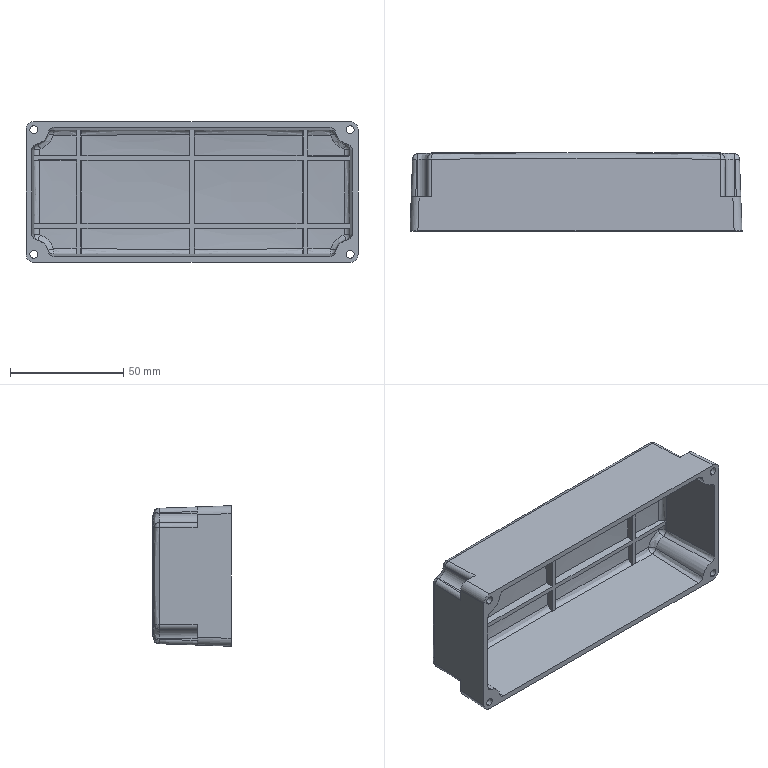Part | NX | features BREP 1 | 1 solid | 176 faces | box 146.5 x 34.5 x 62 mm | volume 53198 mm3 | spline 59 | plane 56 | cylinder 36 | sphere 17 | cone 8 | commonest cylinder face diameters 3.5 x8 4 x8 5 x8 7 x4 8 x4 13 x4